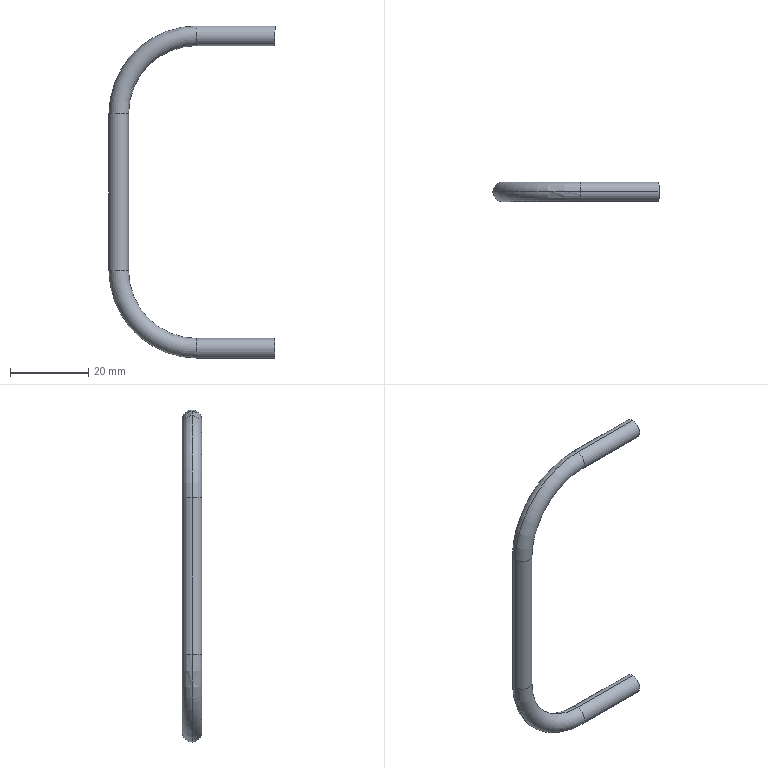Part | SolidWorks | features Sweep 1 | 1 solid | 12 faces | box 42.5 x 5 x 85 mm | volume 2804 mm3 | cylinder 6 | torus 4 | plane 2 | commonest cylinder face diameters 5 x6
STEP:
#1=CARTESIAN_POINT('',(-20.,0.,-2.5));
#2=VERTEX_POINT('',#1);
#3=CARTESIAN_POINT('',(-20.,0.,2.5));
#4=VERTEX_POINT('',#3);
#5=CARTESIAN_POINT('',(-20.,0.,0.));
#6=DIRECTION('',(1.,0.,0.));
#7=DIRECTION('',(0.,0.,-1.));
#8=AXIS2_PLACEMENT_3D('',#5,#6,#7);
#9=CIRCLE('',#8,2.5);
#10=EDGE_CURVE('',#2,#4,#9,.T.);
#11=ORIENTED_EDGE('',*,*,#10,.F.);
#12=CARTESIAN_POINT('',(-42.5,0.,20.));
#13=VERTEX_POINT('',#12);
#14=CARTESIAN_POINT('',(-20.,0.,20.));
#15=DIRECTION('',(0.,1.,0.));
#16=DIRECTION('',(0.,0.,1.));
#17=AXIS2_PLACEMENT_3D('',#14,#15,#16);
#18=CIRCLE('',#17,22.5);
#19=EDGE_CURVE('',#2,#13,#18,.T.);
#20=ORIENTED_EDGE('',*,*,#19,.T.);
#21=CARTESIAN_POINT('',(-37.5,0.,20.));
#22=VERTEX_POINT('',#21);
#23=CARTESIAN_POINT('',(-40.,0.,20.));
#24=DIRECTION('',(0.,0.,-1.));
#25=DIRECTION('',(-1.,0.,0.));
#26=AXIS2_PLACEMENT_3D('',#23,#24,#25);
#27=CIRCLE('',#26,2.5);
#28=EDGE_CURVE('',#13,#22,#27,.T.);
#29=ORIENTED_EDGE('',*,*,#28,.T.);
#30=CARTESIAN_POINT('',(-20.,0.,20.));
#31=DIRECTION('',(0.,1.,0.));
#32=DIRECTION('',(0.,0.,1.));
#33=AXIS2_PLACEMENT_3D('',#30,#31,#32);
#34=CIRCLE('',#33,17.5);
#35=EDGE_CURVE('',#4,#22,#34,.T.);
#36=ORIENTED_EDGE('',*,*,#35,.F.);
#37=EDGE_LOOP('',(#11,#20,#29,#36));
#38=FACE_OUTER_BOUND('',#37,.T.);
#39=CARTESIAN_POINT('',(-20.,0.,20.));
#40=DIRECTION('',(0.,1.,0.));
#41=DIRECTION('',(0.,0.,1.));
#42=AXIS2_PLACEMENT_3D('',#39,#40,#41);
#43=TOROIDAL_SURFACE('',#42,20.,2.5);
#44=ADVANCED_FACE('',(#38),#43,.T.);
#45=CARTESIAN_POINT('',(-42.5,0.,60.));
#46=VERTEX_POINT('',#45);
#47=CARTESIAN_POINT('',(-37.5,0.,60.));
#48=VERTEX_POINT('',#47);
#49=CARTESIAN_POINT('',(-40.,0.,60.));
#50=DIRECTION('',(0.,0.,-1.));
#51=DIRECTION('',(-1.,0.,0.));
#52=AXIS2_PLACEMENT_3D('',#49,#50,#51);
#53=CIRCLE('',#52,2.5);
#54=EDGE_CURVE('',#46,#48,#53,.T.);
#55=ORIENTED_EDGE('',*,*,#54,.F.);
#56=CARTESIAN_POINT('',(-20.,0.,82.5));
#57=VERTEX_POINT('',#56);
#58=CARTESIAN_POINT('',(-20.,0.,60.));
#59=DIRECTION('',(0.,1.,0.));
#60=DIRECTION('',(0.,0.,1.));
#61=AXIS2_PLACEMENT_3D('',#58,#59,#60);
#62=CIRCLE('',#61,22.5);
#63=EDGE_CURVE('',#46,#57,#62,.T.);
#64=ORIENTED_EDGE('',*,*,#63,.T.);
#65=CARTESIAN_POINT('',(-20.,0.,77.5));
#66=VERTEX_POINT('',#65);
#67=CARTESIAN_POINT('',(-20.,0.,80.));
#68=DIRECTION('',(-1.,0.,0.));
#69=DIRECTION('',(0.,0.,1.));
#70=AXIS2_PLACEMENT_3D('',#67,#68,#69);
#71=CIRCLE('',#70,2.5);
#72=EDGE_CURVE('',#57,#66,#71,.T.);
#73=ORIENTED_EDGE('',*,*,#72,.T.);
#74=CARTESIAN_POINT('',(-20.,0.,60.));
#75=DIRECTION('',(0.,1.,0.));
#76=DIRECTION('',(0.,0.,1.));
#77=AXIS2_PLACEMENT_3D('',#74,#75,#76);
#78=CIRCLE('',#77,17.5);
#79=EDGE_CURVE('',#48,#66,#78,.T.);
#80=ORIENTED_EDGE('',*,*,#79,.F.);
#81=EDGE_LOOP('',(#55,#64,#73,#80));
#82=FACE_OUTER_BOUND('',#81,.T.);
#83=CARTESIAN_POINT('',(-20.,0.,60.));
#84=DIRECTION('',(0.,1.,0.));
#85=DIRECTION('',(0.,0.,1.));
#86=AXIS2_PLACEMENT_3D('',#83,#84,#85);
#87=TOROIDAL_SURFACE('',#86,20.,2.5);
#88=ADVANCED_FACE('',(#82),#87,.T.);
#89=ORIENTED_EDGE('',*,*,#10,.T.);
#90=CARTESIAN_POINT('',(0.,0.,2.5));
#91=VERTEX_POINT('',#90);
#92=CARTESIAN_POINT('',(-20.,0.,2.5));
#93=DIRECTION('',(1.,0.,0.));
#94=VECTOR('',#93,1000.);
#95=LINE('',#92,#94);
#96=EDGE_CURVE('',#4,#91,#95,.T.);
#97=ORIENTED_EDGE('',*,*,#96,.T.);
#98=CARTESIAN_POINT('',(0.,0.,-2.5));
#99=VERTEX_POINT('',#98);
#100=CARTESIAN_POINT('',(0.,0.,0.));
#101=DIRECTION('',(1.,0.,0.));
#102=DIRECTION('',(0.,0.,-1.));
#103=AXIS2_PLACEMENT_3D('',#100,#101,#102);
#104=CIRCLE('',#103,2.5);
#105=EDGE_CURVE('',#99,#91,#104,.T.);
#106=ORIENTED_EDGE('',*,*,#105,.F.);
#107=CARTESIAN_POINT('',(-20.,0.,-2.5));
#108=DIRECTION('',(1.,0.,0.));
#109=VECTOR('',#108,1000.);
#110=LINE('',#107,#109);
#111=EDGE_CURVE('',#2,#99,#110,.T.);
#112=ORIENTED_EDGE('',*,*,#111,.F.);
#113=EDGE_LOOP('',(#89,#97,#106,#112));
#114=FACE_OUTER_BOUND('',#113,.T.);
#115=CARTESIAN_POINT('',(-20.,0.,0.));
#116=DIRECTION('',(1.,0.,0.));
#117=DIRECTION('',(0.,0.,-1.));
#118=AXIS2_PLACEMENT_3D('',#115,#116,#117);
#119=CYLINDRICAL_SURFACE('',#118,2.5);
#120=ADVANCED_FACE('',(#114),#119,.T.);
#121=ORIENTED_EDGE('',*,*,#28,.F.);
#122=CARTESIAN_POINT('',(-42.5,0.,20.));
#123=DIRECTION('',(0.,0.,1.));
#124=VECTOR('',#123,1000.);
#125=LINE('',#122,#124);
#126=EDGE_CURVE('',#13,#46,#125,.T.);
#127=ORIENTED_EDGE('',*,*,#126,.T.);
#128=ORIENTED_EDGE('',*,*,#54,.T.);
#129=CARTESIAN_POINT('',(-37.5,0.,20.));
#130=DIRECTION('',(0.,0.,1.));
#131=VECTOR('',#130,1000.);
#132=LINE('',#129,#131);
#133=EDGE_CURVE('',#22,#48,#132,.T.);
#134=ORIENTED_EDGE('',*,*,#133,.F.);
#135=EDGE_LOOP('',(#121,#127,#128,#134));
#136=FACE_OUTER_BOUND('',#135,.T.);
#137=CARTESIAN_POINT('',(-40.,0.,20.));
#138=DIRECTION('',(0.,0.,1.));
#139=DIRECTION('',(1.,0.,0.));
#140=AXIS2_PLACEMENT_3D('',#137,#138,#139);
#141=CYLINDRICAL_SURFACE('',#140,2.5);
#142=ADVANCED_FACE('',(#136),#141,.T.);
#143=ORIENTED_EDGE('',*,*,#72,.F.);
#144=CARTESIAN_POINT('',(0.,0.,82.5));
#145=VERTEX_POINT('',#144);
#146=CARTESIAN_POINT('',(-20.,0.,82.5));
#147=DIRECTION('',(1.,0.,0.));
#148=VECTOR('',#147,1000.);
#149=LINE('',#146,#148);
#150=EDGE_CURVE('',#57,#145,#149,.T.);
#151=ORIENTED_EDGE('',*,*,#150,.T.);
#152=CARTESIAN_POINT('',(0.,0.,77.5));
#153=VERTEX_POINT('',#152);
#154=CARTESIAN_POINT('',(0.,0.,80.));
#155=DIRECTION('',(-1.,0.,0.));
#156=DIRECTION('',(0.,0.,1.));
#157=AXIS2_PLACEMENT_3D('',#154,#155,#156);
#158=CIRCLE('',#157,2.5);
#159=EDGE_CURVE('',#145,#153,#158,.T.);
#160=ORIENTED_EDGE('',*,*,#159,.T.);
#161=CARTESIAN_POINT('',(-20.,0.,77.5));
#162=DIRECTION('',(1.,0.,0.));
#163=VECTOR('',#162,1000.);
#164=LINE('',#161,#163);
#165=EDGE_CURVE('',#66,#153,#164,.T.);
#166=ORIENTED_EDGE('',*,*,#165,.F.);
#167=EDGE_LOOP('',(#143,#151,#160,#166));
#168=FACE_OUTER_BOUND('',#167,.T.);
#169=CARTESIAN_POINT('',(-20.,0.,80.));
#170=DIRECTION('',(1.,0.,0.));
#171=DIRECTION('',(0.,0.,-1.));
#172=AXIS2_PLACEMENT_3D('',#169,#170,#171);
#173=CYLINDRICAL_SURFACE('',#172,2.5);
#174=ADVANCED_FACE('',(#168),#173,.T.);
#175=ORIENTED_EDGE('',*,*,#150,.F.);
#176=CARTESIAN_POINT('',(-20.,0.,80.));
#177=DIRECTION('',(-1.,0.,0.));
#178=DIRECTION('',(0.,0.,1.));
#179=AXIS2_PLACEMENT_3D('',#176,#177,#178);
#180=CIRCLE('',#179,2.5);
#181=EDGE_CURVE('',#66,#57,#180,.T.);
#182=ORIENTED_EDGE('',*,*,#181,.F.);
#183=ORIENTED_EDGE('',*,*,#165,.T.);
#184=CARTESIAN_POINT('',(0.,0.,80.));
#185=DIRECTION('',(-1.,0.,0.));
#186=DIRECTION('',(0.,0.,1.));
#187=AXIS2_PLACEMENT_3D('',#184,#185,#186);
#188=CIRCLE('',#187,2.5);
#189=EDGE_CURVE('',#153,#145,#188,.T.);
#190=ORIENTED_EDGE('',*,*,#189,.T.);
#191=EDGE_LOOP('',(#175,#182,#183,#190));
#192=FACE_OUTER_BOUND('',#191,.T.);
#193=CARTESIAN_POINT('',(-20.,0.,80.));
#194=DIRECTION('',(1.,0.,0.));
#195=DIRECTION('',(0.,0.,-1.));
#196=AXIS2_PLACEMENT_3D('',#193,#194,#195);
#197=CYLINDRICAL_SURFACE('',#196,2.5);
#198=ADVANCED_FACE('',(#192),#197,.T.);
#199=ORIENTED_EDGE('',*,*,#63,.F.);
#200=CARTESIAN_POINT('',(-40.,0.,60.));
#201=DIRECTION('',(0.,0.,-1.));
#202=DIRECTION('',(-1.,0.,0.));
#203=AXIS2_PLACEMENT_3D('',#200,#201,#202);
#204=CIRCLE('',#203,2.5);
#205=EDGE_CURVE('',#48,#46,#204,.T.);
#206=ORIENTED_EDGE('',*,*,#205,.F.);
#207=ORIENTED_EDGE('',*,*,#79,.T.);
#208=ORIENTED_EDGE('',*,*,#181,.T.);
#209=EDGE_LOOP('',(#199,#206,#207,#208));
#210=FACE_OUTER_BOUND('',#209,.T.);
#211=CARTESIAN_POINT('',(-20.,0.,60.));
#212=DIRECTION('',(0.,1.,0.));
#213=DIRECTION('',(0.,0.,1.));
#214=AXIS2_PLACEMENT_3D('',#211,#212,#213);
#215=TOROIDAL_SURFACE('',#214,20.,2.5);
#216=ADVANCED_FACE('',(#210),#215,.T.);
#217=ORIENTED_EDGE('',*,*,#126,.F.);
#218=CARTESIAN_POINT('',(-40.,0.,20.));
#219=DIRECTION('',(0.,0.,-1.));
#220=DIRECTION('',(-1.,0.,0.));
#221=AXIS2_PLACEMENT_3D('',#218,#219,#220);
#222=CIRCLE('',#221,2.5);
#223=EDGE_CURVE('',#22,#13,#222,.T.);
#224=ORIENTED_EDGE('',*,*,#223,.F.);
#225=ORIENTED_EDGE('',*,*,#133,.T.);
#226=ORIENTED_EDGE('',*,*,#205,.T.);
#227=EDGE_LOOP('',(#217,#224,#225,#226));
#228=FACE_OUTER_BOUND('',#227,.T.);
#229=CARTESIAN_POINT('',(-40.,0.,20.));
#230=DIRECTION('',(0.,0.,1.));
#231=DIRECTION('',(1.,0.,0.));
#232=AXIS2_PLACEMENT_3D('',#229,#230,#231);
#233=CYLINDRICAL_SURFACE('',#232,2.5);
#234=ADVANCED_FACE('',(#228),#233,.T.);
#235=ORIENTED_EDGE('',*,*,#19,.F.);
#236=CARTESIAN_POINT('',(-20.,0.,0.));
#237=DIRECTION('',(1.,0.,0.));
#238=DIRECTION('',(0.,0.,-1.));
#239=AXIS2_PLACEMENT_3D('',#236,#237,#238);
#240=CIRCLE('',#239,2.5);
#241=EDGE_CURVE('',#4,#2,#240,.T.);
#242=ORIENTED_EDGE('',*,*,#241,.F.);
#243=ORIENTED_EDGE('',*,*,#35,.T.);
#244=ORIENTED_EDGE('',*,*,#223,.T.);
#245=EDGE_LOOP('',(#235,#242,#243,#244));
#246=FACE_OUTER_BOUND('',#245,.T.);
#247=CARTESIAN_POINT('',(-20.,0.,20.));
#248=DIRECTION('',(0.,1.,0.));
#249=DIRECTION('',(0.,0.,1.));
#250=AXIS2_PLACEMENT_3D('',#247,#248,#249);
#251=TOROIDAL_SURFACE('',#250,20.,2.5);
#252=ADVANCED_FACE('',(#246),#251,.T.);
#253=ORIENTED_EDGE('',*,*,#96,.F.);
#254=ORIENTED_EDGE('',*,*,#241,.T.);
#255=ORIENTED_EDGE('',*,*,#111,.T.);
#256=CARTESIAN_POINT('',(0.,0.,0.));
#257=DIRECTION('',(1.,0.,0.));
#258=DIRECTION('',(0.,0.,-1.));
#259=AXIS2_PLACEMENT_3D('',#256,#257,#258);
#260=CIRCLE('',#259,2.5);
#261=EDGE_CURVE('',#91,#99,#260,.T.);
#262=ORIENTED_EDGE('',*,*,#261,.F.);
#263=EDGE_LOOP('',(#253,#254,#255,#262));
#264=FACE_OUTER_BOUND('',#263,.T.);
#265=CARTESIAN_POINT('',(-20.,0.,0.));
#266=DIRECTION('',(1.,0.,0.));
#267=DIRECTION('',(0.,0.,-1.));
#268=AXIS2_PLACEMENT_3D('',#265,#266,#267);
#269=CYLINDRICAL_SURFACE('',#268,2.5);
#270=ADVANCED_FACE('',(#264),#269,.T.);
#271=ORIENTED_EDGE('',*,*,#189,.F.);
#272=ORIENTED_EDGE('',*,*,#159,.F.);
#273=EDGE_LOOP('',(#271,#272));
#274=FACE_OUTER_BOUND('',#273,.T.);
#275=CARTESIAN_POINT('',(0.,0.,80.));
#276=DIRECTION('',(-1.,0.,0.));
#277=DIRECTION('',(0.,0.,1.));
#278=AXIS2_PLACEMENT_3D('',#275,#276,#277);
#279=PLANE('',#278);
#280=ADVANCED_FACE('',(#274),#279,.F.);
#281=ORIENTED_EDGE('',*,*,#105,.T.);
#282=ORIENTED_EDGE('',*,*,#261,.T.);
#283=EDGE_LOOP('',(#281,#282));
#284=FACE_OUTER_BOUND('',#283,.T.);
#285=CARTESIAN_POINT('',(0.,0.,0.));
#286=DIRECTION('',(1.,0.,0.));
#287=DIRECTION('',(0.,0.,-1.));
#288=AXIS2_PLACEMENT_3D('',#285,#286,#287);
#289=PLANE('',#288);
#290=ADVANCED_FACE('',(#284),#289,.T.);
#291=CLOSED_SHELL('',(#44,#88,#120,#142,#174,#198,#216,#234,#252,#270,#280,#290));
#292=MANIFOLD_SOLID_BREP('',#291);
#293=CARTESIAN_POINT('',(0.,0.,0.));
#294=DIRECTION('',(0.,0.,1.));
#295=DIRECTION('',(1.,0.,0.));
#296=AXIS2_PLACEMENT_3D('',#293,#294,#295);
#297=(LENGTH_UNIT()NAMED_UNIT(*)SI_UNIT(.MILLI.,.METRE.));
#298=UNCERTAINTY_MEASURE_WITH_UNIT(LENGTH_MEASURE(0.00001),#297,'','');
#299=(NAMED_UNIT(*)PLANE_ANGLE_UNIT()SI_UNIT($,.RADIAN.));
#300=(NAMED_UNIT(*)SI_UNIT($,.STERADIAN.)SOLID_ANGLE_UNIT());
#301=(GEOMETRIC_REPRESENTATION_CONTEXT(3)GLOBAL_UNCERTAINTY_ASSIGNED_CONTEXT((#298))GLOBAL_UNIT_ASSIGNED_CONTEXT((#297,#299,#300))REPRESENTATION_CONTEXT('',''));
#302=ADVANCED_BREP_SHAPE_REPRESENTATION('',(#292,#296),#301);